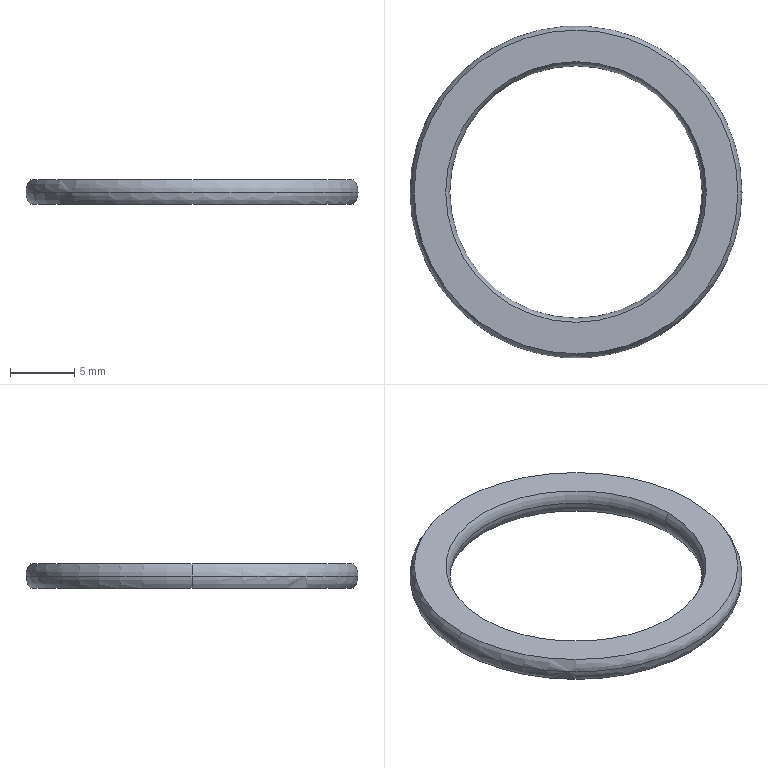Part | Creo | 1 solid | 10 faces | box 25.8 x 25.8 x 1.9 mm | volume 392.015 mm3 | torus 8 | plane 2
STEP:
#1=CARTESIAN_POINT('',(65.875,-41.,-105.));
#2=VERTEX_POINT('',#1);
#3=CARTESIAN_POINT('',(86.125,-41.,-105.));
#4=VERTEX_POINT('',#3);
#5=CARTESIAN_POINT('',(76.,-41.,-105.));
#6=DIRECTION('',(0.,0.,-1.));
#7=DIRECTION('',(-1.,0.,0.));
#8=AXIS2_PLACEMENT_3D('',#5,#6,#7);
#9=CIRCLE('',#8,10.125);
#10=EDGE_CURVE('',#2,#4,#9,.T.);
#11=ORIENTED_EDGE('',*,*,#10,.T.);
#12=CARTESIAN_POINT('',(85.8,-41.,-105.95));
#13=VERTEX_POINT('',#12);
#14=CARTESIAN_POINT('',(87.35,-41.,-105.95));
#15=DIRECTION('',(0.,1.,0.));
#16=DIRECTION('',(-1.,0.,0.));
#17=AXIS2_PLACEMENT_3D('',#14,#15,#16);
#18=CIRCLE('',#17,1.55);
#19=EDGE_CURVE('',#13,#4,#18,.T.);
#20=ORIENTED_EDGE('',*,*,#19,.F.);
#21=CARTESIAN_POINT('',(66.2,-41.,-105.95));
#22=VERTEX_POINT('',#21);
#23=CARTESIAN_POINT('',(76.,-41.,-105.95));
#24=DIRECTION('',(0.,0.,-1.));
#25=DIRECTION('',(-1.,0.,0.));
#26=AXIS2_PLACEMENT_3D('',#23,#24,#25);
#27=CIRCLE('',#26,9.8);
#28=EDGE_CURVE('',#22,#13,#27,.T.);
#29=ORIENTED_EDGE('',*,*,#28,.F.);
#30=CARTESIAN_POINT('',(64.65,-41.,-105.95));
#31=DIRECTION('',(0.,-1.,0.));
#32=DIRECTION('',(1.,0.,0.));
#33=AXIS2_PLACEMENT_3D('',#30,#31,#32);
#34=CIRCLE('',#33,1.55);
#35=EDGE_CURVE('',#22,#2,#34,.T.);
#36=ORIENTED_EDGE('',*,*,#35,.T.);
#37=EDGE_LOOP('',(#11,#20,#29,#36));
#38=FACE_OUTER_BOUND('',#37,.F.);
#39=CARTESIAN_POINT('',(76.,-41.,-105.95));
#40=DIRECTION('',(0.,0.,-1.));
#41=DIRECTION('',(-1.,0.,0.));
#42=AXIS2_PLACEMENT_3D('',#39,#40,#41);
#43=TOROIDAL_SURFACE('',#42,11.35,1.55);
#44=ADVANCED_FACE('',(#38),#43,.T.);
#45=CARTESIAN_POINT('',(63.425,-41.,-105.));
#46=VERTEX_POINT('',#45);
#47=CARTESIAN_POINT('',(88.575,-41.,-105.));
#48=VERTEX_POINT('',#47);
#49=CARTESIAN_POINT('',(76.,-41.,-105.));
#50=DIRECTION('',(0.,0.,1.));
#51=DIRECTION('',(-1.,0.,0.));
#52=AXIS2_PLACEMENT_3D('',#49,#50,#51);
#53=CIRCLE('',#52,12.575);
#54=EDGE_CURVE('',#46,#48,#53,.T.);
#55=ORIENTED_EDGE('',*,*,#54,.F.);
#56=CARTESIAN_POINT('',(76.,-41.,-105.));
#57=DIRECTION('',(0.,0.,1.));
#58=DIRECTION('',(1.,0.,0.));
#59=AXIS2_PLACEMENT_3D('',#56,#57,#58);
#60=CIRCLE('',#59,12.575);
#61=EDGE_CURVE('',#48,#46,#60,.T.);
#62=ORIENTED_EDGE('',*,*,#61,.F.);
#63=EDGE_LOOP('',(#55,#62));
#64=FACE_OUTER_BOUND('',#63,.F.);
#65=ORIENTED_EDGE('',*,*,#10,.F.);
#66=CARTESIAN_POINT('',(76.,-41.,-105.));
#67=DIRECTION('',(0.,0.,-1.));
#68=DIRECTION('',(1.,0.,0.));
#69=AXIS2_PLACEMENT_3D('',#66,#67,#68);
#70=CIRCLE('',#69,10.125);
#71=EDGE_CURVE('',#4,#2,#70,.T.);
#72=ORIENTED_EDGE('',*,*,#71,.F.);
#73=EDGE_LOOP('',(#65,#72));
#74=FACE_BOUND('',#73,.F.);
#75=CARTESIAN_POINT('',(76.,-28.425,-105.));
#76=DIRECTION('',(0.,0.,1.));
#77=DIRECTION('',(1.,0.,0.));
#78=AXIS2_PLACEMENT_3D('',#75,#76,#77);
#79=PLANE('',#78);
#80=ADVANCED_FACE('',(#64,#74),#79,.T.);
#81=ORIENTED_EDGE('',*,*,#71,.T.);
#82=ORIENTED_EDGE('',*,*,#35,.F.);
#83=CARTESIAN_POINT('',(76.,-41.,-105.95));
#84=DIRECTION('',(0.,0.,-1.));
#85=DIRECTION('',(1.,0.,0.));
#86=AXIS2_PLACEMENT_3D('',#83,#84,#85);
#87=CIRCLE('',#86,9.8);
#88=EDGE_CURVE('',#13,#22,#87,.T.);
#89=ORIENTED_EDGE('',*,*,#88,.F.);
#90=ORIENTED_EDGE('',*,*,#19,.T.);
#91=EDGE_LOOP('',(#81,#82,#89,#90));
#92=FACE_OUTER_BOUND('',#91,.F.);
#93=CARTESIAN_POINT('',(76.,-41.,-105.95));
#94=DIRECTION('',(0.,0.,-1.));
#95=DIRECTION('',(-1.,0.,0.));
#96=AXIS2_PLACEMENT_3D('',#93,#94,#95);
#97=TOROIDAL_SURFACE('',#96,11.35,1.55);
#98=ADVANCED_FACE('',(#92),#97,.T.);
#99=CARTESIAN_POINT('',(65.875,-41.,-106.9));
#100=VERTEX_POINT('',#99);
#101=CARTESIAN_POINT('',(86.125,-41.,-106.9));
#102=VERTEX_POINT('',#101);
#103=CARTESIAN_POINT('',(76.,-41.,-106.9));
#104=DIRECTION('',(0.,0.,1.));
#105=DIRECTION('',(-1.,0.,0.));
#106=AXIS2_PLACEMENT_3D('',#103,#104,#105);
#107=CIRCLE('',#106,10.125);
#108=EDGE_CURVE('',#100,#102,#107,.T.);
#109=ORIENTED_EDGE('',*,*,#108,.T.);
#110=CARTESIAN_POINT('',(87.35,-41.,-105.95));
#111=DIRECTION('',(0.,1.,0.));
#112=DIRECTION('',(-0.7902,0.,-0.6129));
#113=AXIS2_PLACEMENT_3D('',#110,#111,#112);
#114=CIRCLE('',#113,1.55);
#115=EDGE_CURVE('',#102,#13,#114,.T.);
#116=ORIENTED_EDGE('',*,*,#115,.T.);
#117=ORIENTED_EDGE('',*,*,#88,.T.);
#118=CARTESIAN_POINT('',(64.65,-41.,-105.95));
#119=DIRECTION('',(0.,-1.,0.));
#120=DIRECTION('',(0.7902,0.,-0.6129));
#121=AXIS2_PLACEMENT_3D('',#118,#119,#120);
#122=CIRCLE('',#121,1.55);
#123=EDGE_CURVE('',#100,#22,#122,.T.);
#124=ORIENTED_EDGE('',*,*,#123,.F.);
#125=EDGE_LOOP('',(#109,#116,#117,#124));
#126=FACE_OUTER_BOUND('',#125,.F.);
#127=CARTESIAN_POINT('',(76.,-41.,-105.95));
#128=DIRECTION('',(0.,0.,-1.));
#129=DIRECTION('',(-1.,0.,0.));
#130=AXIS2_PLACEMENT_3D('',#127,#128,#129);
#131=TOROIDAL_SURFACE('',#130,11.35,1.55);
#132=ADVANCED_FACE('',(#126),#131,.T.);
#133=CARTESIAN_POINT('',(63.425,-41.,-106.9));
#134=VERTEX_POINT('',#133);
#135=CARTESIAN_POINT('',(88.575,-41.,-106.9));
#136=VERTEX_POINT('',#135);
#137=CARTESIAN_POINT('',(76.,-41.,-106.9));
#138=DIRECTION('',(0.,0.,-1.));
#139=DIRECTION('',(-1.,0.,0.));
#140=AXIS2_PLACEMENT_3D('',#137,#138,#139);
#141=CIRCLE('',#140,12.575);
#142=EDGE_CURVE('',#134,#136,#141,.T.);
#143=ORIENTED_EDGE('',*,*,#142,.F.);
#144=CARTESIAN_POINT('',(76.,-41.,-106.9));
#145=DIRECTION('',(0.,0.,-1.));
#146=DIRECTION('',(1.,0.,0.));
#147=AXIS2_PLACEMENT_3D('',#144,#145,#146);
#148=CIRCLE('',#147,12.575);
#149=EDGE_CURVE('',#136,#134,#148,.T.);
#150=ORIENTED_EDGE('',*,*,#149,.F.);
#151=EDGE_LOOP('',(#143,#150));
#152=FACE_OUTER_BOUND('',#151,.F.);
#153=ORIENTED_EDGE('',*,*,#108,.F.);
#154=CARTESIAN_POINT('',(76.,-41.,-106.9));
#155=DIRECTION('',(0.,0.,1.));
#156=DIRECTION('',(1.,0.,0.));
#157=AXIS2_PLACEMENT_3D('',#154,#155,#156);
#158=CIRCLE('',#157,10.125);
#159=EDGE_CURVE('',#102,#100,#158,.T.);
#160=ORIENTED_EDGE('',*,*,#159,.F.);
#161=EDGE_LOOP('',(#153,#160));
#162=FACE_BOUND('',#161,.F.);
#163=CARTESIAN_POINT('',(76.,-30.875,-106.9));
#164=DIRECTION('',(0.,0.,-1.));
#165=DIRECTION('',(-1.,0.,0.));
#166=AXIS2_PLACEMENT_3D('',#163,#164,#165);
#167=PLANE('',#166);
#168=ADVANCED_FACE('',(#152,#162),#167,.T.);
#169=ORIENTED_EDGE('',*,*,#142,.T.);
#170=CARTESIAN_POINT('',(88.9,-41.,-105.95));
#171=VERTEX_POINT('',#170);
#172=CARTESIAN_POINT('',(87.35,-41.,-105.95));
#173=DIRECTION('',(0.,1.,0.));
#174=DIRECTION('',(1.,0.,0.));
#175=AXIS2_PLACEMENT_3D('',#172,#173,#174);
#176=CIRCLE('',#175,1.55);
#177=EDGE_CURVE('',#171,#136,#176,.T.);
#178=ORIENTED_EDGE('',*,*,#177,.F.);
#179=CARTESIAN_POINT('',(63.1,-41.,-105.95));
#180=VERTEX_POINT('',#179);
#181=CARTESIAN_POINT('',(76.,-41.,-105.95));
#182=DIRECTION('',(0.,0.,-1.));
#183=DIRECTION('',(-1.,0.,0.));
#184=AXIS2_PLACEMENT_3D('',#181,#182,#183);
#185=CIRCLE('',#184,12.9);
#186=EDGE_CURVE('',#180,#171,#185,.T.);
#187=ORIENTED_EDGE('',*,*,#186,.F.);
#188=CARTESIAN_POINT('',(64.65,-41.,-105.95));
#189=DIRECTION('',(0.,-1.,0.));
#190=DIRECTION('',(-1.,0.,0.));
#191=AXIS2_PLACEMENT_3D('',#188,#189,#190);
#192=CIRCLE('',#191,1.55);
#193=EDGE_CURVE('',#180,#134,#192,.T.);
#194=ORIENTED_EDGE('',*,*,#193,.T.);
#195=EDGE_LOOP('',(#169,#178,#187,#194));
#196=FACE_OUTER_BOUND('',#195,.F.);
#197=CARTESIAN_POINT('',(76.,-41.,-105.95));
#198=DIRECTION('',(0.,0.,-1.));
#199=DIRECTION('',(-1.,0.,0.));
#200=AXIS2_PLACEMENT_3D('',#197,#198,#199);
#201=TOROIDAL_SURFACE('',#200,11.35,1.55);
#202=ADVANCED_FACE('',(#196),#201,.T.);
#203=ORIENTED_EDGE('',*,*,#149,.T.);
#204=ORIENTED_EDGE('',*,*,#193,.F.);
#205=CARTESIAN_POINT('',(76.,-41.,-105.95));
#206=DIRECTION('',(0.,0.,-1.));
#207=DIRECTION('',(1.,0.,0.));
#208=AXIS2_PLACEMENT_3D('',#205,#206,#207);
#209=CIRCLE('',#208,12.9);
#210=EDGE_CURVE('',#171,#180,#209,.T.);
#211=ORIENTED_EDGE('',*,*,#210,.F.);
#212=ORIENTED_EDGE('',*,*,#177,.T.);
#213=EDGE_LOOP('',(#203,#204,#211,#212));
#214=FACE_OUTER_BOUND('',#213,.F.);
#215=CARTESIAN_POINT('',(76.,-41.,-105.95));
#216=DIRECTION('',(0.,0.,-1.));
#217=DIRECTION('',(-1.,0.,0.));
#218=AXIS2_PLACEMENT_3D('',#215,#216,#217);
#219=TOROIDAL_SURFACE('',#218,11.35,1.55);
#220=ADVANCED_FACE('',(#214),#219,.T.);
#221=ORIENTED_EDGE('',*,*,#54,.T.);
#222=CARTESIAN_POINT('',(87.35,-41.,-105.95));
#223=DIRECTION('',(0.,1.,0.));
#224=DIRECTION('',(0.7902,0.,0.6129));
#225=AXIS2_PLACEMENT_3D('',#222,#223,#224);
#226=CIRCLE('',#225,1.55);
#227=EDGE_CURVE('',#48,#171,#226,.T.);
#228=ORIENTED_EDGE('',*,*,#227,.T.);
#229=ORIENTED_EDGE('',*,*,#210,.T.);
#230=CARTESIAN_POINT('',(64.65,-41.,-105.95));
#231=DIRECTION('',(0.,-1.,0.));
#232=DIRECTION('',(-0.7902,0.,0.6129));
#233=AXIS2_PLACEMENT_3D('',#230,#231,#232);
#234=CIRCLE('',#233,1.55);
#235=EDGE_CURVE('',#46,#180,#234,.T.);
#236=ORIENTED_EDGE('',*,*,#235,.F.);
#237=EDGE_LOOP('',(#221,#228,#229,#236));
#238=FACE_OUTER_BOUND('',#237,.F.);
#239=CARTESIAN_POINT('',(76.,-41.,-105.95));
#240=DIRECTION('',(0.,0.,-1.));
#241=DIRECTION('',(-1.,0.,0.));
#242=AXIS2_PLACEMENT_3D('',#239,#240,#241);
#243=TOROIDAL_SURFACE('',#242,11.35,1.55);
#244=ADVANCED_FACE('',(#238),#243,.T.);
#245=ORIENTED_EDGE('',*,*,#61,.T.);
#246=ORIENTED_EDGE('',*,*,#235,.T.);
#247=ORIENTED_EDGE('',*,*,#186,.T.);
#248=ORIENTED_EDGE('',*,*,#227,.F.);
#249=EDGE_LOOP('',(#245,#246,#247,#248));
#250=FACE_OUTER_BOUND('',#249,.F.);
#251=CARTESIAN_POINT('',(76.,-41.,-105.95));
#252=DIRECTION('',(0.,0.,-1.));
#253=DIRECTION('',(-1.,0.,0.));
#254=AXIS2_PLACEMENT_3D('',#251,#252,#253);
#255=TOROIDAL_SURFACE('',#254,11.35,1.55);
#256=ADVANCED_FACE('',(#250),#255,.T.);
#257=ORIENTED_EDGE('',*,*,#159,.T.);
#258=ORIENTED_EDGE('',*,*,#123,.T.);
#259=ORIENTED_EDGE('',*,*,#28,.T.);
#260=ORIENTED_EDGE('',*,*,#115,.F.);
#261=EDGE_LOOP('',(#257,#258,#259,#260));
#262=FACE_OUTER_BOUND('',#261,.F.);
#263=CARTESIAN_POINT('',(76.,-41.,-105.95));
#264=DIRECTION('',(0.,0.,-1.));
#265=DIRECTION('',(-1.,0.,0.));
#266=AXIS2_PLACEMENT_3D('',#263,#264,#265);
#267=TOROIDAL_SURFACE('',#266,11.35,1.55);
#268=ADVANCED_FACE('',(#262),#267,.T.);
#269=CLOSED_SHELL('',(#44,#80,#98,#132,#168,#202,#220,#244,#256,#268));
#270=MANIFOLD_SOLID_BREP('',#269);
#271=(LENGTH_UNIT()NAMED_UNIT(*)SI_UNIT(.MILLI.,.METRE.));
#272=UNCERTAINTY_MEASURE_WITH_UNIT(LENGTH_MEASURE(0.003653),#271,'','');
#273=(NAMED_UNIT(*)PLANE_ANGLE_UNIT()SI_UNIT($,.RADIAN.));
#274=PLANE_ANGLE_MEASURE_WITH_UNIT(PLANE_ANGLE_MEASURE(0.01745),#273);
#275=(CONVERSION_BASED_UNIT('DEGREE',#274)NAMED_UNIT(*)PLANE_ANGLE_UNIT());
#276=(NAMED_UNIT(*)SI_UNIT($,.STERADIAN.)SOLID_ANGLE_UNIT());
#277=(GEOMETRIC_REPRESENTATION_CONTEXT(3)GLOBAL_UNCERTAINTY_ASSIGNED_CONTEXT((#272))GLOBAL_UNIT_ASSIGNED_CONTEXT((#271,#275,#276))REPRESENTATION_CONTEXT('',''));
#278=ADVANCED_BREP_SHAPE_REPRESENTATION('',(#270),#277);